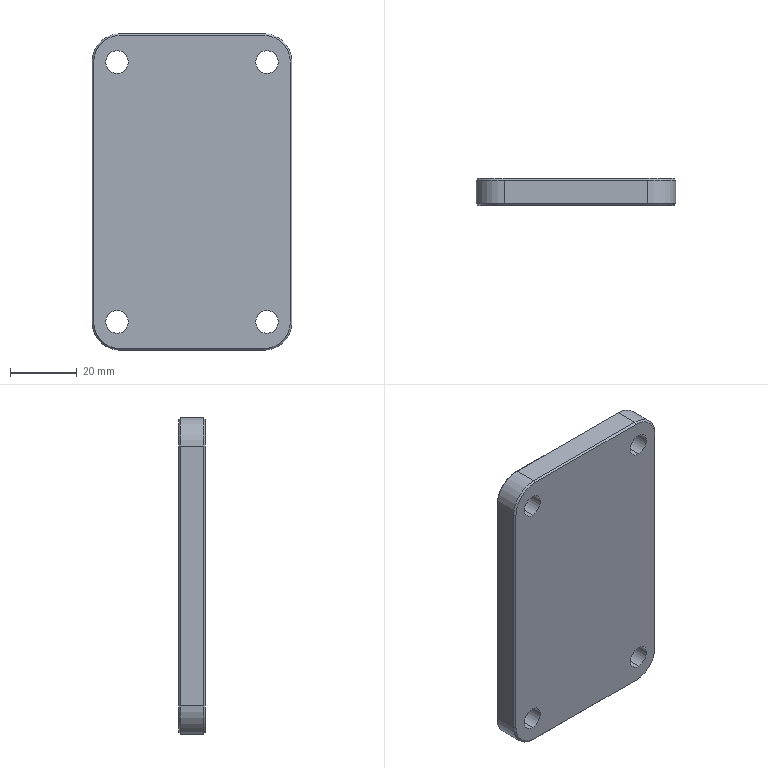Part | SolidWorks | features Chamfer 1, Extrusion 1, Fillet 1, HoleWzd 1 | 1 solid | 34 faces | box 60 x 8 x 95 mm | volume 43868 mm3 | plane 14 | cylinder 12 | cone 8 | commonest cylinder face diameters 6.8 x8 17 x4
STEP:
#1=CARTESIAN_POINT('',(-22.5,0.,-38.1));
#2=VERTEX_POINT('',#1);
#3=CARTESIAN_POINT('',(-22.5,0.,-44.9));
#4=VERTEX_POINT('',#3);
#5=CARTESIAN_POINT('',(-22.5,0.,-41.5));
#6=DIRECTION('',(0.,-1.,0.));
#7=DIRECTION('',(0.,0.,-1.));
#8=AXIS2_PLACEMENT_3D('',#5,#6,#7);
#9=CIRCLE('',#8,3.4);
#10=EDGE_CURVE('',#2,#4,#9,.T.);
#11=ORIENTED_EDGE('',*,*,#10,.F.);
#12=CARTESIAN_POINT('',(-22.5,-8.,-38.1));
#13=VERTEX_POINT('',#12);
#14=CARTESIAN_POINT('',(-22.5,-8.,-38.1));
#15=DIRECTION('',(0.,-1.,0.));
#16=VECTOR('',#15,1000.);
#17=LINE('',#14,#16);
#18=EDGE_CURVE('',#2,#13,#17,.T.);
#19=ORIENTED_EDGE('',*,*,#18,.T.);
#20=CARTESIAN_POINT('',(-22.5,-8.,-44.9));
#21=VERTEX_POINT('',#20);
#22=CARTESIAN_POINT('',(-22.5,-8.,-41.5));
#23=DIRECTION('',(0.,-1.,0.));
#24=DIRECTION('',(0.,0.,-1.));
#25=AXIS2_PLACEMENT_3D('',#22,#23,#24);
#26=CIRCLE('',#25,3.4);
#27=EDGE_CURVE('',#13,#21,#26,.T.);
#28=ORIENTED_EDGE('',*,*,#27,.T.);
#29=CARTESIAN_POINT('',(-22.5,-8.,-44.9));
#30=DIRECTION('',(0.,-1.,0.));
#31=VECTOR('',#30,1000.);
#32=LINE('',#29,#31);
#33=EDGE_CURVE('',#4,#21,#32,.T.);
#34=ORIENTED_EDGE('',*,*,#33,.F.);
#35=EDGE_LOOP('',(#11,#19,#28,#34));
#36=FACE_OUTER_BOUND('',#35,.T.);
#37=CARTESIAN_POINT('',(-22.5,-8.,-41.5));
#38=DIRECTION('',(0.,-1.,0.));
#39=DIRECTION('',(0.,0.,-1.));
#40=AXIS2_PLACEMENT_3D('',#37,#38,#39);
#41=CYLINDRICAL_SURFACE('',#40,3.4);
#42=ADVANCED_FACE('',(#36),#41,.F.);
#43=CARTESIAN_POINT('',(22.5,0.,-38.1));
#44=VERTEX_POINT('',#43);
#45=CARTESIAN_POINT('',(22.5,0.,-44.9));
#46=VERTEX_POINT('',#45);
#47=CARTESIAN_POINT('',(22.5,0.,-41.5));
#48=DIRECTION('',(0.,-1.,0.));
#49=DIRECTION('',(0.,0.,-1.));
#50=AXIS2_PLACEMENT_3D('',#47,#48,#49);
#51=CIRCLE('',#50,3.4);
#52=EDGE_CURVE('',#44,#46,#51,.T.);
#53=ORIENTED_EDGE('',*,*,#52,.F.);
#54=CARTESIAN_POINT('',(22.5,-8.,-38.1));
#55=VERTEX_POINT('',#54);
#56=CARTESIAN_POINT('',(22.5,-8.,-38.1));
#57=DIRECTION('',(0.,-1.,0.));
#58=VECTOR('',#57,1000.);
#59=LINE('',#56,#58);
#60=EDGE_CURVE('',#44,#55,#59,.T.);
#61=ORIENTED_EDGE('',*,*,#60,.T.);
#62=CARTESIAN_POINT('',(22.5,-8.,-44.9));
#63=VERTEX_POINT('',#62);
#64=CARTESIAN_POINT('',(22.5,-8.,-41.5));
#65=DIRECTION('',(0.,-1.,0.));
#66=DIRECTION('',(0.,0.,-1.));
#67=AXIS2_PLACEMENT_3D('',#64,#65,#66);
#68=CIRCLE('',#67,3.4);
#69=EDGE_CURVE('',#55,#63,#68,.T.);
#70=ORIENTED_EDGE('',*,*,#69,.T.);
#71=CARTESIAN_POINT('',(22.5,-8.,-44.9));
#72=DIRECTION('',(0.,-1.,0.));
#73=VECTOR('',#72,1000.);
#74=LINE('',#71,#73);
#75=EDGE_CURVE('',#46,#63,#74,.T.);
#76=ORIENTED_EDGE('',*,*,#75,.F.);
#77=EDGE_LOOP('',(#53,#61,#70,#76));
#78=FACE_OUTER_BOUND('',#77,.T.);
#79=CARTESIAN_POINT('',(22.5,-8.,-41.5));
#80=DIRECTION('',(0.,-1.,0.));
#81=DIRECTION('',(0.,0.,-1.));
#82=AXIS2_PLACEMENT_3D('',#79,#80,#81);
#83=CYLINDRICAL_SURFACE('',#82,3.4);
#84=ADVANCED_FACE('',(#78),#83,.F.);
#85=CARTESIAN_POINT('',(22.5,0.,39.9));
#86=VERTEX_POINT('',#85);
#87=CARTESIAN_POINT('',(22.5,0.,33.1));
#88=VERTEX_POINT('',#87);
#89=CARTESIAN_POINT('',(22.5,0.,36.5));
#90=DIRECTION('',(0.,-1.,0.));
#91=DIRECTION('',(0.,0.,-1.));
#92=AXIS2_PLACEMENT_3D('',#89,#90,#91);
#93=CIRCLE('',#92,3.4);
#94=EDGE_CURVE('',#86,#88,#93,.T.);
#95=ORIENTED_EDGE('',*,*,#94,.F.);
#96=CARTESIAN_POINT('',(22.5,-8.,39.9));
#97=VERTEX_POINT('',#96);
#98=CARTESIAN_POINT('',(22.5,-8.,39.9));
#99=DIRECTION('',(0.,-1.,0.));
#100=VECTOR('',#99,1000.);
#101=LINE('',#98,#100);
#102=EDGE_CURVE('',#86,#97,#101,.T.);
#103=ORIENTED_EDGE('',*,*,#102,.T.);
#104=CARTESIAN_POINT('',(22.5,-8.,33.1));
#105=VERTEX_POINT('',#104);
#106=CARTESIAN_POINT('',(22.5,-8.,36.5));
#107=DIRECTION('',(0.,-1.,0.));
#108=DIRECTION('',(0.,0.,-1.));
#109=AXIS2_PLACEMENT_3D('',#106,#107,#108);
#110=CIRCLE('',#109,3.4);
#111=EDGE_CURVE('',#97,#105,#110,.T.);
#112=ORIENTED_EDGE('',*,*,#111,.T.);
#113=CARTESIAN_POINT('',(22.5,-8.,33.1));
#114=DIRECTION('',(0.,-1.,0.));
#115=VECTOR('',#114,1000.);
#116=LINE('',#113,#115);
#117=EDGE_CURVE('',#88,#105,#116,.T.);
#118=ORIENTED_EDGE('',*,*,#117,.F.);
#119=EDGE_LOOP('',(#95,#103,#112,#118));
#120=FACE_OUTER_BOUND('',#119,.T.);
#121=CARTESIAN_POINT('',(22.5,-8.,36.5));
#122=DIRECTION('',(0.,-1.,0.));
#123=DIRECTION('',(0.,0.,-1.));
#124=AXIS2_PLACEMENT_3D('',#121,#122,#123);
#125=CYLINDRICAL_SURFACE('',#124,3.4);
#126=ADVANCED_FACE('',(#120),#125,.F.);
#127=CARTESIAN_POINT('',(-22.5,0.,39.9));
#128=VERTEX_POINT('',#127);
#129=CARTESIAN_POINT('',(-22.5,0.,33.1));
#130=VERTEX_POINT('',#129);
#131=CARTESIAN_POINT('',(-22.5,0.,36.5));
#132=DIRECTION('',(0.,-1.,0.));
#133=DIRECTION('',(0.,0.,-1.));
#134=AXIS2_PLACEMENT_3D('',#131,#132,#133);
#135=CIRCLE('',#134,3.4);
#136=EDGE_CURVE('',#128,#130,#135,.T.);
#137=ORIENTED_EDGE('',*,*,#136,.F.);
#138=CARTESIAN_POINT('',(-22.5,-8.,39.9));
#139=VERTEX_POINT('',#138);
#140=CARTESIAN_POINT('',(-22.5,-8.,39.9));
#141=DIRECTION('',(0.,-1.,0.));
#142=VECTOR('',#141,1000.);
#143=LINE('',#140,#142);
#144=EDGE_CURVE('',#128,#139,#143,.T.);
#145=ORIENTED_EDGE('',*,*,#144,.T.);
#146=CARTESIAN_POINT('',(-22.5,-8.,33.1));
#147=VERTEX_POINT('',#146);
#148=CARTESIAN_POINT('',(-22.5,-8.,36.5));
#149=DIRECTION('',(0.,-1.,0.));
#150=DIRECTION('',(0.,0.,-1.));
#151=AXIS2_PLACEMENT_3D('',#148,#149,#150);
#152=CIRCLE('',#151,3.4);
#153=EDGE_CURVE('',#139,#147,#152,.T.);
#154=ORIENTED_EDGE('',*,*,#153,.T.);
#155=CARTESIAN_POINT('',(-22.5,-8.,33.1));
#156=DIRECTION('',(0.,-1.,0.));
#157=VECTOR('',#156,1000.);
#158=LINE('',#155,#157);
#159=EDGE_CURVE('',#130,#147,#158,.T.);
#160=ORIENTED_EDGE('',*,*,#159,.F.);
#161=EDGE_LOOP('',(#137,#145,#154,#160));
#162=FACE_OUTER_BOUND('',#161,.T.);
#163=CARTESIAN_POINT('',(-22.5,-8.,36.5));
#164=DIRECTION('',(0.,-1.,0.));
#165=DIRECTION('',(0.,0.,-1.));
#166=AXIS2_PLACEMENT_3D('',#163,#164,#165);
#167=CYLINDRICAL_SURFACE('',#166,3.4);
#168=ADVANCED_FACE('',(#162),#167,.F.);
#169=CARTESIAN_POINT('',(-30.,-7.5,36.5));
#170=VERTEX_POINT('',#169);
#171=CARTESIAN_POINT('',(-30.,-0.5,36.5));
#172=VERTEX_POINT('',#171);
#173=CARTESIAN_POINT('',(-30.,0.,36.5));
#174=DIRECTION('',(0.,1.,0.));
#175=VECTOR('',#174,1000.);
#176=LINE('',#173,#175);
#177=EDGE_CURVE('',#170,#172,#176,.T.);
#178=ORIENTED_EDGE('',*,*,#177,.T.);
#179=CARTESIAN_POINT('',(-30.,-0.5,-41.5));
#180=VERTEX_POINT('',#179);
#181=CARTESIAN_POINT('',(-30.,-0.5,-41.5));
#182=DIRECTION('',(0.,0.,-1.));
#183=VECTOR('',#182,1000.);
#184=LINE('',#181,#183);
#185=EDGE_CURVE('',#172,#180,#184,.T.);
#186=ORIENTED_EDGE('',*,*,#185,.T.);
#187=CARTESIAN_POINT('',(-30.,-7.5,-41.5));
#188=VERTEX_POINT('',#187);
#189=CARTESIAN_POINT('',(-30.,0.,-41.5));
#190=DIRECTION('',(0.,-1.,0.));
#191=VECTOR('',#190,1000.);
#192=LINE('',#189,#191);
#193=EDGE_CURVE('',#180,#188,#192,.T.);
#194=ORIENTED_EDGE('',*,*,#193,.T.);
#195=CARTESIAN_POINT('',(-30.,-7.5,45.));
#196=DIRECTION('',(0.,0.,1.));
#197=VECTOR('',#196,1000.);
#198=LINE('',#195,#197);
#199=EDGE_CURVE('',#188,#170,#198,.T.);
#200=ORIENTED_EDGE('',*,*,#199,.T.);
#201=EDGE_LOOP('',(#178,#186,#194,#200));
#202=FACE_OUTER_BOUND('',#201,.T.);
#203=CARTESIAN_POINT('',(-30.,0.,45.));
#204=DIRECTION('',(-1.,0.,0.));
#205=DIRECTION('',(0.,0.,1.));
#206=AXIS2_PLACEMENT_3D('',#203,#204,#205);
#207=PLANE('',#206);
#208=ADVANCED_FACE('',(#202),#207,.T.);
#209=CARTESIAN_POINT('',(21.5,-7.5,45.));
#210=VERTEX_POINT('',#209);
#211=CARTESIAN_POINT('',(21.5,-0.5,45.));
#212=VERTEX_POINT('',#211);
#213=CARTESIAN_POINT('',(21.5,0.,45.));
#214=DIRECTION('',(0.,1.,0.));
#215=VECTOR('',#214,1000.);
#216=LINE('',#213,#215);
#217=EDGE_CURVE('',#210,#212,#216,.T.);
#218=ORIENTED_EDGE('',*,*,#217,.T.);
#219=CARTESIAN_POINT('',(-21.5,-0.5,45.));
#220=VERTEX_POINT('',#219);
#221=CARTESIAN_POINT('',(-21.5,-0.5,45.));
#222=DIRECTION('',(-1.,0.,0.));
#223=VECTOR('',#222,1000.);
#224=LINE('',#221,#223);
#225=EDGE_CURVE('',#212,#220,#224,.T.);
#226=ORIENTED_EDGE('',*,*,#225,.T.);
#227=CARTESIAN_POINT('',(-21.5,-7.5,45.));
#228=VERTEX_POINT('',#227);
#229=CARTESIAN_POINT('',(-21.5,0.,45.));
#230=DIRECTION('',(0.,-1.,0.));
#231=VECTOR('',#230,1000.);
#232=LINE('',#229,#231);
#233=EDGE_CURVE('',#220,#228,#232,.T.);
#234=ORIENTED_EDGE('',*,*,#233,.T.);
#235=CARTESIAN_POINT('',(30.,-7.5,45.));
#236=DIRECTION('',(1.,0.,0.));
#237=VECTOR('',#236,1000.);
#238=LINE('',#235,#237);
#239=EDGE_CURVE('',#228,#210,#238,.T.);
#240=ORIENTED_EDGE('',*,*,#239,.T.);
#241=EDGE_LOOP('',(#218,#226,#234,#240));
#242=FACE_OUTER_BOUND('',#241,.T.);
#243=CARTESIAN_POINT('',(30.,0.,45.));
#244=DIRECTION('',(0.,0.,1.));
#245=DIRECTION('',(1.,0.,0.));
#246=AXIS2_PLACEMENT_3D('',#243,#244,#245);
#247=PLANE('',#246);
#248=ADVANCED_FACE('',(#242),#247,.T.);
#249=CARTESIAN_POINT('',(30.,-7.5,-41.5));
#250=VERTEX_POINT('',#249);
#251=CARTESIAN_POINT('',(30.,-0.5,-41.5));
#252=VERTEX_POINT('',#251);
#253=CARTESIAN_POINT('',(30.,0.,-41.5));
#254=DIRECTION('',(0.,1.,0.));
#255=VECTOR('',#254,1000.);
#256=LINE('',#253,#255);
#257=EDGE_CURVE('',#250,#252,#256,.T.);
#258=ORIENTED_EDGE('',*,*,#257,.T.);
#259=CARTESIAN_POINT('',(30.,-0.5,36.5));
#260=VERTEX_POINT('',#259);
#261=CARTESIAN_POINT('',(30.,-0.5,36.5));
#262=DIRECTION('',(0.,0.,1.));
#263=VECTOR('',#262,1000.);
#264=LINE('',#261,#263);
#265=EDGE_CURVE('',#252,#260,#264,.T.);
#266=ORIENTED_EDGE('',*,*,#265,.T.);
#267=CARTESIAN_POINT('',(30.,-7.5,36.5));
#268=VERTEX_POINT('',#267);
#269=CARTESIAN_POINT('',(30.,0.,36.5));
#270=DIRECTION('',(0.,-1.,0.));
#271=VECTOR('',#270,1000.);
#272=LINE('',#269,#271);
#273=EDGE_CURVE('',#260,#268,#272,.T.);
#274=ORIENTED_EDGE('',*,*,#273,.T.);
#275=CARTESIAN_POINT('',(30.,-7.5,-50.));
#276=DIRECTION('',(0.,0.,-1.));
#277=VECTOR('',#276,1000.);
#278=LINE('',#275,#277);
#279=EDGE_CURVE('',#268,#250,#278,.T.);
#280=ORIENTED_EDGE('',*,*,#279,.T.);
#281=EDGE_LOOP('',(#258,#266,#274,#280));
#282=FACE_OUTER_BOUND('',#281,.T.);
#283=CARTESIAN_POINT('',(30.,0.,-50.));
#284=DIRECTION('',(1.,0.,0.));
#285=DIRECTION('',(0.,0.,-1.));
#286=AXIS2_PLACEMENT_3D('',#283,#284,#285);
#287=PLANE('',#286);
#288=ADVANCED_FACE('',(#282),#287,.T.);
#289=CARTESIAN_POINT('',(-21.5,-7.5,-50.));
#290=VERTEX_POINT('',#289);
#291=CARTESIAN_POINT('',(-21.5,-0.5,-50.));
#292=VERTEX_POINT('',#291);
#293=CARTESIAN_POINT('',(-21.5,0.,-50.));
#294=DIRECTION('',(0.,1.,0.));
#295=VECTOR('',#294,1000.);
#296=LINE('',#293,#295);
#297=EDGE_CURVE('',#290,#292,#296,.T.);
#298=ORIENTED_EDGE('',*,*,#297,.T.);
#299=CARTESIAN_POINT('',(21.5,-0.5,-50.));
#300=VERTEX_POINT('',#299);
#301=CARTESIAN_POINT('',(21.5,-0.5,-50.));
#302=DIRECTION('',(1.,0.,0.));
#303=VECTOR('',#302,1000.);
#304=LINE('',#301,#303);
#305=EDGE_CURVE('',#292,#300,#304,.T.);
#306=ORIENTED_EDGE('',*,*,#305,.T.);
#307=CARTESIAN_POINT('',(21.5,-7.5,-50.));
#308=VERTEX_POINT('',#307);
#309=CARTESIAN_POINT('',(21.5,0.,-50.));
#310=DIRECTION('',(0.,-1.,0.));
#311=VECTOR('',#310,1000.);
#312=LINE('',#309,#311);
#313=EDGE_CURVE('',#300,#308,#312,.T.);
#314=ORIENTED_EDGE('',*,*,#313,.T.);
#315=CARTESIAN_POINT('',(-30.,-7.5,-50.));
#316=DIRECTION('',(-1.,0.,0.));
#317=VECTOR('',#316,1000.);
#318=LINE('',#315,#317);
#319=EDGE_CURVE('',#308,#290,#318,.T.);
#320=ORIENTED_EDGE('',*,*,#319,.T.);
#321=EDGE_LOOP('',(#298,#306,#314,#320));
#322=FACE_OUTER_BOUND('',#321,.T.);
#323=CARTESIAN_POINT('',(-30.,0.,-50.));
#324=DIRECTION('',(0.,0.,-1.));
#325=DIRECTION('',(-1.,0.,0.));
#326=AXIS2_PLACEMENT_3D('',#323,#324,#325);
#327=PLANE('',#326);
#328=ADVANCED_FACE('',(#322),#327,.T.);
#329=CARTESIAN_POINT('',(21.5,0.,44.5));
#330=VERTEX_POINT('',#329);
#331=CARTESIAN_POINT('',(29.5,0.,36.5));
#332=VERTEX_POINT('',#331);
#333=CARTESIAN_POINT('',(21.5,0.,36.5));
#334=DIRECTION('',(0.,1.,0.));
#335=DIRECTION('',(0.,0.,-1.));
#336=AXIS2_PLACEMENT_3D('',#333,#334,#335);
#337=CIRCLE('',#336,8.);
#338=EDGE_CURVE('',#330,#332,#337,.T.);
#339=ORIENTED_EDGE('',*,*,#338,.T.);
#340=CARTESIAN_POINT('',(29.5,0.,-41.5));
#341=VERTEX_POINT('',#340);
#342=CARTESIAN_POINT('',(29.5,0.,-41.5));
#343=DIRECTION('',(0.,0.,-1.));
#344=VECTOR('',#343,1000.);
#345=LINE('',#342,#344);
#346=EDGE_CURVE('',#332,#341,#345,.T.);
#347=ORIENTED_EDGE('',*,*,#346,.T.);
#348=CARTESIAN_POINT('',(21.5,0.,-49.5));
#349=VERTEX_POINT('',#348);
#350=CARTESIAN_POINT('',(21.5,0.,-41.5));
#351=DIRECTION('',(0.,1.,0.));
#352=DIRECTION('',(0.,0.,-1.));
#353=AXIS2_PLACEMENT_3D('',#350,#351,#352);
#354=CIRCLE('',#353,8.);
#355=EDGE_CURVE('',#341,#349,#354,.T.);
#356=ORIENTED_EDGE('',*,*,#355,.T.);
#357=CARTESIAN_POINT('',(-21.5,0.,-49.5));
#358=VERTEX_POINT('',#357);
#359=CARTESIAN_POINT('',(-21.5,0.,-49.5));
#360=DIRECTION('',(-1.,0.,0.));
#361=VECTOR('',#360,1000.);
#362=LINE('',#359,#361);
#363=EDGE_CURVE('',#349,#358,#362,.T.);
#364=ORIENTED_EDGE('',*,*,#363,.T.);
#365=CARTESIAN_POINT('',(-29.5,0.,-41.5));
#366=VERTEX_POINT('',#365);
#367=CARTESIAN_POINT('',(-21.5,0.,-41.5));
#368=DIRECTION('',(0.,1.,0.));
#369=DIRECTION('',(0.,0.,-1.));
#370=AXIS2_PLACEMENT_3D('',#367,#368,#369);
#371=CIRCLE('',#370,8.);
#372=EDGE_CURVE('',#358,#366,#371,.T.);
#373=ORIENTED_EDGE('',*,*,#372,.T.);
#374=CARTESIAN_POINT('',(-29.5,0.,36.5));
#375=VERTEX_POINT('',#374);
#376=CARTESIAN_POINT('',(-29.5,0.,36.5));
#377=DIRECTION('',(0.,0.,1.));
#378=VECTOR('',#377,1000.);
#379=LINE('',#376,#378);
#380=EDGE_CURVE('',#366,#375,#379,.T.);
#381=ORIENTED_EDGE('',*,*,#380,.T.);
#382=CARTESIAN_POINT('',(-21.5,0.,44.5));
#383=VERTEX_POINT('',#382);
#384=CARTESIAN_POINT('',(-21.5,0.,36.5));
#385=DIRECTION('',(0.,1.,0.));
#386=DIRECTION('',(0.,0.,-1.));
#387=AXIS2_PLACEMENT_3D('',#384,#385,#386);
#388=CIRCLE('',#387,8.);
#389=EDGE_CURVE('',#375,#383,#388,.T.);
#390=ORIENTED_EDGE('',*,*,#389,.T.);
#391=CARTESIAN_POINT('',(21.5,0.,44.5));
#392=DIRECTION('',(1.,0.,0.));
#393=VECTOR('',#392,1000.);
#394=LINE('',#391,#393);
#395=EDGE_CURVE('',#383,#330,#394,.T.);
#396=ORIENTED_EDGE('',*,*,#395,.T.);
#397=EDGE_LOOP('',(#339,#347,#356,#364,#373,#381,#390,#396));
#398=FACE_OUTER_BOUND('',#397,.T.);
#399=CARTESIAN_POINT('',(-22.5,0.,-41.5));
#400=DIRECTION('',(0.,-1.,0.));
#401=DIRECTION('',(0.,0.,-1.));
#402=AXIS2_PLACEMENT_3D('',#399,#400,#401);
#403=CIRCLE('',#402,3.4);
#404=EDGE_CURVE('',#4,#2,#403,.T.);
#405=ORIENTED_EDGE('',*,*,#404,.T.);
#406=ORIENTED_EDGE('',*,*,#10,.T.);
#407=EDGE_LOOP('',(#405,#406));
#408=FACE_BOUND('',#407,.T.);
#409=CARTESIAN_POINT('',(22.5,0.,-41.5));
#410=DIRECTION('',(0.,-1.,0.));
#411=DIRECTION('',(0.,0.,-1.));
#412=AXIS2_PLACEMENT_3D('',#409,#410,#411);
#413=CIRCLE('',#412,3.4);
#414=EDGE_CURVE('',#46,#44,#413,.T.);
#415=ORIENTED_EDGE('',*,*,#414,.T.);
#416=ORIENTED_EDGE('',*,*,#52,.T.);
#417=EDGE_LOOP('',(#415,#416));
#418=FACE_BOUND('',#417,.T.);
#419=CARTESIAN_POINT('',(22.5,0.,36.5));
#420=DIRECTION('',(0.,-1.,0.));
#421=DIRECTION('',(0.,0.,-1.));
#422=AXIS2_PLACEMENT_3D('',#419,#420,#421);
#423=CIRCLE('',#422,3.4);
#424=EDGE_CURVE('',#88,#86,#423,.T.);
#425=ORIENTED_EDGE('',*,*,#424,.T.);
#426=ORIENTED_EDGE('',*,*,#94,.T.);
#427=EDGE_LOOP('',(#425,#426));
#428=FACE_BOUND('',#427,.T.);
#429=CARTESIAN_POINT('',(-22.5,0.,36.5));
#430=DIRECTION('',(0.,-1.,0.));
#431=DIRECTION('',(0.,0.,-1.));
#432=AXIS2_PLACEMENT_3D('',#429,#430,#431);
#433=CIRCLE('',#432,3.4);
#434=EDGE_CURVE('',#130,#128,#433,.T.);
#435=ORIENTED_EDGE('',*,*,#434,.T.);
#436=ORIENTED_EDGE('',*,*,#136,.T.);
#437=EDGE_LOOP('',(#435,#436));
#438=FACE_BOUND('',#437,.T.);
#439=CARTESIAN_POINT('',(0.,0.,0.));
#440=DIRECTION('',(0.,-1.,0.));
#441=DIRECTION('',(0.,0.,-1.));
#442=AXIS2_PLACEMENT_3D('',#439,#440,#441);
#443=PLANE('',#442);
#444=ADVANCED_FACE('',(#398,#408,#418,#428,#438),#443,.F.);
#445=CARTESIAN_POINT('',(21.5,-8.,44.5));
#446=VERTEX_POINT('',#445);
#447=CARTESIAN_POINT('',(-21.5,-8.,44.5));
#448=VERTEX_POINT('',#447);
#449=CARTESIAN_POINT('',(0.,-8.,44.5));
#450=DIRECTION('',(-1.,0.,0.));
#451=VECTOR('',#450,1000.);
#452=LINE('',#449,#451);
#453=EDGE_CURVE('',#446,#448,#452,.T.);
#454=ORIENTED_EDGE('',*,*,#453,.T.);
#455=CARTESIAN_POINT('',(-29.5,-8.,36.5));
#456=VERTEX_POINT('',#455);
#457=CARTESIAN_POINT('',(-21.5,-8.,36.5));
#458=DIRECTION('',(0.,-1.,0.));
#459=DIRECTION('',(0.,0.,-1.));
#460=AXIS2_PLACEMENT_3D('',#457,#458,#459);
#461=CIRCLE('',#460,8.);
#462=EDGE_CURVE('',#448,#456,#461,.T.);
#463=ORIENTED_EDGE('',*,*,#462,.T.);
#464=CARTESIAN_POINT('',(-29.5,-8.,-41.5));
#465=VERTEX_POINT('',#464);
#466=CARTESIAN_POINT('',(-29.5,-8.,0.));
#467=DIRECTION('',(0.,0.,-1.));
#468=VECTOR('',#467,1000.);
#469=LINE('',#466,#468);
#470=EDGE_CURVE('',#456,#465,#469,.T.);
#471=ORIENTED_EDGE('',*,*,#470,.T.);
#472=CARTESIAN_POINT('',(-21.5,-8.,-49.5));
#473=VERTEX_POINT('',#472);
#474=CARTESIAN_POINT('',(-21.5,-8.,-41.5));
#475=DIRECTION('',(0.,-1.,0.));
#476=DIRECTION('',(0.,0.,-1.));
#477=AXIS2_PLACEMENT_3D('',#474,#475,#476);
#478=CIRCLE('',#477,8.);
#479=EDGE_CURVE('',#465,#473,#478,.T.);
#480=ORIENTED_EDGE('',*,*,#479,.T.);
#481=CARTESIAN_POINT('',(21.5,-8.,-49.5));
#482=VERTEX_POINT('',#481);
#483=CARTESIAN_POINT('',(0.,-8.,-49.5));
#484=DIRECTION('',(1.,0.,0.));
#485=VECTOR('',#484,1000.);
#486=LINE('',#483,#485);
#487=EDGE_CURVE('',#473,#482,#486,.T.);
#488=ORIENTED_EDGE('',*,*,#487,.T.);
#489=CARTESIAN_POINT('',(29.5,-8.,-41.5));
#490=VERTEX_POINT('',#489);
#491=CARTESIAN_POINT('',(21.5,-8.,-41.5));
#492=DIRECTION('',(0.,-1.,0.));
#493=DIRECTION('',(0.,0.,-1.));
#494=AXIS2_PLACEMENT_3D('',#491,#492,#493);
#495=CIRCLE('',#494,8.);
#496=EDGE_CURVE('',#482,#490,#495,.T.);
#497=ORIENTED_EDGE('',*,*,#496,.T.);
#498=CARTESIAN_POINT('',(29.5,-8.,36.5));
#499=VERTEX_POINT('',#498);
#500=CARTESIAN_POINT('',(29.5,-8.,0.));
#501=DIRECTION('',(0.,0.,1.));
#502=VECTOR('',#501,1000.);
#503=LINE('',#500,#502);
#504=EDGE_CURVE('',#490,#499,#503,.T.);
#505=ORIENTED_EDGE('',*,*,#504,.T.);
#506=CARTESIAN_POINT('',(21.5,-8.,36.5));
#507=DIRECTION('',(0.,-1.,0.));
#508=DIRECTION('',(0.,0.,-1.));
#509=AXIS2_PLACEMENT_3D('',#506,#507,#508);
#510=CIRCLE('',#509,8.);
#511=EDGE_CURVE('',#499,#446,#510,.T.);
#512=ORIENTED_EDGE('',*,*,#511,.T.);
#513=EDGE_LOOP('',(#454,#463,#471,#480,#488,#497,#505,#512));
#514=FACE_OUTER_BOUND('',#513,.T.);
#515=CARTESIAN_POINT('',(-22.5,-8.,-41.5));
#516=DIRECTION('',(0.,-1.,0.));
#517=DIRECTION('',(0.,0.,-1.));
#518=AXIS2_PLACEMENT_3D('',#515,#516,#517);
#519=CIRCLE('',#518,3.4);
#520=EDGE_CURVE('',#21,#13,#519,.T.);
#521=ORIENTED_EDGE('',*,*,#520,.F.);
#522=ORIENTED_EDGE('',*,*,#27,.F.);
#523=EDGE_LOOP('',(#521,#522));
#524=FACE_BOUND('',#523,.T.);
#525=CARTESIAN_POINT('',(22.5,-8.,-41.5));
#526=DIRECTION('',(0.,-1.,0.));
#527=DIRECTION('',(0.,0.,-1.));
#528=AXIS2_PLACEMENT_3D('',#525,#526,#527);
#529=CIRCLE('',#528,3.4);
#530=EDGE_CURVE('',#63,#55,#529,.T.);
#531=ORIENTED_EDGE('',*,*,#530,.F.);
#532=ORIENTED_EDGE('',*,*,#69,.F.);
#533=EDGE_LOOP('',(#531,#532));
#534=FACE_BOUND('',#533,.T.);
#535=CARTESIAN_POINT('',(22.5,-8.,36.5));
#536=DIRECTION('',(0.,-1.,0.));
#537=DIRECTION('',(0.,0.,-1.));
#538=AXIS2_PLACEMENT_3D('',#535,#536,#537);
#539=CIRCLE('',#538,3.4);
#540=EDGE_CURVE('',#105,#97,#539,.T.);
#541=ORIENTED_EDGE('',*,*,#540,.F.);
#542=ORIENTED_EDGE('',*,*,#111,.F.);
#543=EDGE_LOOP('',(#541,#542));
#544=FACE_BOUND('',#543,.T.);
#545=CARTESIAN_POINT('',(-22.5,-8.,36.5));
#546=DIRECTION('',(0.,-1.,0.));
#547=DIRECTION('',(0.,0.,-1.));
#548=AXIS2_PLACEMENT_3D('',#545,#546,#547);
#549=CIRCLE('',#548,3.4);
#550=EDGE_CURVE('',#147,#139,#549,.T.);
#551=ORIENTED_EDGE('',*,*,#550,.F.);
#552=ORIENTED_EDGE('',*,*,#153,.F.);
#553=EDGE_LOOP('',(#551,#552));
#554=FACE_BOUND('',#553,.T.);
#555=CARTESIAN_POINT('',(0.,-8.,0.));
#556=DIRECTION('',(0.,-1.,0.));
#557=DIRECTION('',(0.,0.,-1.));
#558=AXIS2_PLACEMENT_3D('',#555,#556,#557);
#559=PLANE('',#558);
#560=ADVANCED_FACE('',(#514,#524,#534,#544,#554),#559,.T.);
#561=ORIENTED_EDGE('',*,*,#144,.F.);
#562=ORIENTED_EDGE('',*,*,#434,.F.);
#563=ORIENTED_EDGE('',*,*,#159,.T.);
#564=ORIENTED_EDGE('',*,*,#550,.T.);
#565=EDGE_LOOP('',(#561,#562,#563,#564));
#566=FACE_OUTER_BOUND('',#565,.T.);
#567=CARTESIAN_POINT('',(-22.5,-8.,36.5));
#568=DIRECTION('',(0.,-1.,0.));
#569=DIRECTION('',(0.,0.,-1.));
#570=AXIS2_PLACEMENT_3D('',#567,#568,#569);
#571=CYLINDRICAL_SURFACE('',#570,3.4);
#572=ADVANCED_FACE('',(#566),#571,.F.);
#573=ORIENTED_EDGE('',*,*,#102,.F.);
#574=ORIENTED_EDGE('',*,*,#424,.F.);
#575=ORIENTED_EDGE('',*,*,#117,.T.);
#576=ORIENTED_EDGE('',*,*,#540,.T.);
#577=EDGE_LOOP('',(#573,#574,#575,#576));
#578=FACE_OUTER_BOUND('',#577,.T.);
#579=CARTESIAN_POINT('',(22.5,-8.,36.5));
#580=DIRECTION('',(0.,-1.,0.));
#581=DIRECTION('',(0.,0.,-1.));
#582=AXIS2_PLACEMENT_3D('',#579,#580,#581);
#583=CYLINDRICAL_SURFACE('',#582,3.4);
#584=ADVANCED_FACE('',(#578),#583,.F.);
#585=ORIENTED_EDGE('',*,*,#60,.F.);
#586=ORIENTED_EDGE('',*,*,#414,.F.);
#587=ORIENTED_EDGE('',*,*,#75,.T.);
#588=ORIENTED_EDGE('',*,*,#530,.T.);
#589=EDGE_LOOP('',(#585,#586,#587,#588));
#590=FACE_OUTER_BOUND('',#589,.T.);
#591=CARTESIAN_POINT('',(22.5,-8.,-41.5));
#592=DIRECTION('',(0.,-1.,0.));
#593=DIRECTION('',(0.,0.,-1.));
#594=AXIS2_PLACEMENT_3D('',#591,#592,#593);
#595=CYLINDRICAL_SURFACE('',#594,3.4);
#596=ADVANCED_FACE('',(#590),#595,.F.);
#597=ORIENTED_EDGE('',*,*,#18,.F.);
#598=ORIENTED_EDGE('',*,*,#404,.F.);
#599=ORIENTED_EDGE('',*,*,#33,.T.);
#600=ORIENTED_EDGE('',*,*,#520,.T.);
#601=EDGE_LOOP('',(#597,#598,#599,#600));
#602=FACE_OUTER_BOUND('',#601,.T.);
#603=CARTESIAN_POINT('',(-22.5,-8.,-41.5));
#604=DIRECTION('',(0.,-1.,0.));
#605=DIRECTION('',(0.,0.,-1.));
#606=AXIS2_PLACEMENT_3D('',#603,#604,#605);
#607=CYLINDRICAL_SURFACE('',#606,3.4);
#608=ADVANCED_FACE('',(#602),#607,.F.);
#609=ORIENTED_EDGE('',*,*,#313,.F.);
#610=CARTESIAN_POINT('',(21.5,-0.5,-41.5));
#611=DIRECTION('',(0.,-1.,0.));
#612=DIRECTION('',(0.,0.,-1.));
#613=AXIS2_PLACEMENT_3D('',#610,#611,#612);
#614=CIRCLE('',#613,8.5);
#615=EDGE_CURVE('',#300,#252,#614,.T.);
#616=ORIENTED_EDGE('',*,*,#615,.T.);
#617=ORIENTED_EDGE('',*,*,#257,.F.);
#618=CARTESIAN_POINT('',(21.5,-7.5,-41.5));
#619=DIRECTION('',(0.,1.,0.));
#620=DIRECTION('',(0.,0.,-1.));
#621=AXIS2_PLACEMENT_3D('',#618,#619,#620);
#622=CIRCLE('',#621,8.5);
#623=EDGE_CURVE('',#250,#308,#622,.T.);
#624=ORIENTED_EDGE('',*,*,#623,.T.);
#625=EDGE_LOOP('',(#609,#616,#617,#624));
#626=FACE_OUTER_BOUND('',#625,.T.);
#627=CARTESIAN_POINT('',(21.5,0.,-41.5));
#628=DIRECTION('',(0.,-1.,0.));
#629=DIRECTION('',(0.,0.,-1.));
#630=AXIS2_PLACEMENT_3D('',#627,#628,#629);
#631=CYLINDRICAL_SURFACE('',#630,8.5);
#632=ADVANCED_FACE('',(#626),#631,.T.);
#633=ORIENTED_EDGE('',*,*,#273,.F.);
#634=CARTESIAN_POINT('',(21.5,-0.5,36.5));
#635=DIRECTION('',(0.,-1.,0.));
#636=DIRECTION('',(0.,0.,-1.));
#637=AXIS2_PLACEMENT_3D('',#634,#635,#636);
#638=CIRCLE('',#637,8.5);
#639=EDGE_CURVE('',#260,#212,#638,.T.);
#640=ORIENTED_EDGE('',*,*,#639,.T.);
#641=ORIENTED_EDGE('',*,*,#217,.F.);
#642=CARTESIAN_POINT('',(21.5,-7.5,36.5));
#643=DIRECTION('',(0.,1.,0.));
#644=DIRECTION('',(0.,0.,-1.));
#645=AXIS2_PLACEMENT_3D('',#642,#643,#644);
#646=CIRCLE('',#645,8.5);
#647=EDGE_CURVE('',#210,#268,#646,.T.);
#648=ORIENTED_EDGE('',*,*,#647,.T.);
#649=EDGE_LOOP('',(#633,#640,#641,#648));
#650=FACE_OUTER_BOUND('',#649,.T.);
#651=CARTESIAN_POINT('',(21.5,0.,36.5));
#652=DIRECTION('',(0.,-1.,0.));
#653=DIRECTION('',(0.,0.,-1.));
#654=AXIS2_PLACEMENT_3D('',#651,#652,#653);
#655=CYLINDRICAL_SURFACE('',#654,8.5);
#656=ADVANCED_FACE('',(#650),#655,.T.);
#657=ORIENTED_EDGE('',*,*,#193,.F.);
#658=CARTESIAN_POINT('',(-21.5,-0.5,-41.5));
#659=DIRECTION('',(0.,-1.,0.));
#660=DIRECTION('',(0.,0.,-1.));
#661=AXIS2_PLACEMENT_3D('',#658,#659,#660);
#662=CIRCLE('',#661,8.5);
#663=EDGE_CURVE('',#180,#292,#662,.T.);
#664=ORIENTED_EDGE('',*,*,#663,.T.);
#665=ORIENTED_EDGE('',*,*,#297,.F.);
#666=CARTESIAN_POINT('',(-21.5,-7.5,-41.5));
#667=DIRECTION('',(0.,1.,0.));
#668=DIRECTION('',(0.,0.,-1.));
#669=AXIS2_PLACEMENT_3D('',#666,#667,#668);
#670=CIRCLE('',#669,8.5);
#671=EDGE_CURVE('',#290,#188,#670,.T.);
#672=ORIENTED_EDGE('',*,*,#671,.T.);
#673=EDGE_LOOP('',(#657,#664,#665,#672));
#674=FACE_OUTER_BOUND('',#673,.T.);
#675=CARTESIAN_POINT('',(-21.5,0.,-41.5));
#676=DIRECTION('',(0.,-1.,0.));
#677=DIRECTION('',(0.,0.,-1.));
#678=AXIS2_PLACEMENT_3D('',#675,#676,#677);
#679=CYLINDRICAL_SURFACE('',#678,8.5);
#680=ADVANCED_FACE('',(#674),#679,.T.);
#681=ORIENTED_EDGE('',*,*,#233,.F.);
#682=CARTESIAN_POINT('',(-21.5,-0.5,36.5));
#683=DIRECTION('',(0.,-1.,0.));
#684=DIRECTION('',(0.,0.,-1.));
#685=AXIS2_PLACEMENT_3D('',#682,#683,#684);
#686=CIRCLE('',#685,8.5);
#687=EDGE_CURVE('',#220,#172,#686,.T.);
#688=ORIENTED_EDGE('',*,*,#687,.T.);
#689=ORIENTED_EDGE('',*,*,#177,.F.);
#690=CARTESIAN_POINT('',(-21.5,-7.5,36.5));
#691=DIRECTION('',(0.,1.,0.));
#692=DIRECTION('',(0.,0.,-1.));
#693=AXIS2_PLACEMENT_3D('',#690,#691,#692);
#694=CIRCLE('',#693,8.5);
#695=EDGE_CURVE('',#170,#228,#694,.T.);
#696=ORIENTED_EDGE('',*,*,#695,.T.);
#697=EDGE_LOOP('',(#681,#688,#689,#696));
#698=FACE_OUTER_BOUND('',#697,.T.);
#699=CARTESIAN_POINT('',(-21.5,0.,36.5));
#700=DIRECTION('',(0.,-1.,0.));
#701=DIRECTION('',(0.,0.,-1.));
#702=AXIS2_PLACEMENT_3D('',#699,#700,#701);
#703=CYLINDRICAL_SURFACE('',#702,8.5);
#704=ADVANCED_FACE('',(#698),#703,.T.);
#705=CARTESIAN_POINT('',(-29.5,0.,36.5));
#706=DIRECTION('',(-0.7071,-0.7071,0.));
#707=VECTOR('',#706,1000.);
#708=LINE('',#705,#707);
#709=EDGE_CURVE('',#375,#172,#708,.T.);
#710=ORIENTED_EDGE('',*,*,#709,.F.);
#711=ORIENTED_EDGE('',*,*,#380,.F.);
#712=CARTESIAN_POINT('',(-30.,-0.5,-41.5));
#713=DIRECTION('',(0.7071,0.7071,0.));
#714=VECTOR('',#713,1000.);
#715=LINE('',#712,#714);
#716=EDGE_CURVE('',#180,#366,#715,.T.);
#717=ORIENTED_EDGE('',*,*,#716,.F.);
#718=ORIENTED_EDGE('',*,*,#185,.F.);
#719=EDGE_LOOP('',(#710,#711,#717,#718));
#720=FACE_OUTER_BOUND('',#719,.T.);
#721=CARTESIAN_POINT('',(-30.,-0.5,45.));
#722=DIRECTION('',(-0.7071,0.7071,0.));
#723=DIRECTION('',(0.,0.,1.));
#724=AXIS2_PLACEMENT_3D('',#721,#722,#723);
#725=PLANE('',#724);
#726=ADVANCED_FACE('',(#720),#725,.T.);
#727=ORIENTED_EDGE('',*,*,#716,.T.);
#728=ORIENTED_EDGE('',*,*,#372,.F.);
#729=CARTESIAN_POINT('',(-21.5,-0.5,-50.));
#730=DIRECTION('',(0.,0.7071,0.7071));
#731=VECTOR('',#730,1000.);
#732=LINE('',#729,#731);
#733=EDGE_CURVE('',#292,#358,#732,.T.);
#734=ORIENTED_EDGE('',*,*,#733,.F.);
#735=ORIENTED_EDGE('',*,*,#663,.F.);
#736=EDGE_LOOP('',(#727,#728,#734,#735));
#737=FACE_OUTER_BOUND('',#736,.T.);
#738=CARTESIAN_POINT('',(-21.5,0.,-41.5));
#739=DIRECTION('',(0.,-1.,0.));
#740=DIRECTION('',(0.,0.,-1.));
#741=AXIS2_PLACEMENT_3D('',#738,#739,#740);
#742=CONICAL_SURFACE('',#741,8.,0.7854);
#743=ADVANCED_FACE('',(#737),#742,.T.);
#744=ORIENTED_EDGE('',*,*,#709,.T.);
#745=ORIENTED_EDGE('',*,*,#687,.F.);
#746=CARTESIAN_POINT('',(-21.5,0.,44.5));
#747=DIRECTION('',(0.,-0.7071,0.7071));
#748=VECTOR('',#747,1000.);
#749=LINE('',#746,#748);
#750=EDGE_CURVE('',#383,#220,#749,.T.);
#751=ORIENTED_EDGE('',*,*,#750,.F.);
#752=ORIENTED_EDGE('',*,*,#389,.F.);
#753=EDGE_LOOP('',(#744,#745,#751,#752));
#754=FACE_OUTER_BOUND('',#753,.T.);
#755=CARTESIAN_POINT('',(-21.5,0.,36.5));
#756=DIRECTION('',(0.,-1.,0.));
#757=DIRECTION('',(0.,0.,-1.));
#758=AXIS2_PLACEMENT_3D('',#755,#756,#757);
#759=CONICAL_SURFACE('',#758,8.,0.7854);
#760=ADVANCED_FACE('',(#754),#759,.T.);
#761=ORIENTED_EDGE('',*,*,#733,.T.);
#762=ORIENTED_EDGE('',*,*,#363,.F.);
#763=CARTESIAN_POINT('',(21.5,-0.5,-50.));
#764=DIRECTION('',(0.,0.7071,0.7071));
#765=VECTOR('',#764,1000.);
#766=LINE('',#763,#765);
#767=EDGE_CURVE('',#300,#349,#766,.T.);
#768=ORIENTED_EDGE('',*,*,#767,.F.);
#769=ORIENTED_EDGE('',*,*,#305,.F.);
#770=EDGE_LOOP('',(#761,#762,#768,#769));
#771=FACE_OUTER_BOUND('',#770,.T.);
#772=CARTESIAN_POINT('',(-30.,-0.5,-50.));
#773=DIRECTION('',(0.,0.7071,-0.7071));
#774=DIRECTION('',(-1.,0.,0.));
#775=AXIS2_PLACEMENT_3D('',#772,#773,#774);
#776=PLANE('',#775);
#777=ADVANCED_FACE('',(#771),#776,.T.);
#778=ORIENTED_EDGE('',*,*,#750,.T.);
#779=ORIENTED_EDGE('',*,*,#225,.F.);
#780=CARTESIAN_POINT('',(21.5,0.,44.5));
#781=DIRECTION('',(0.,-0.7071,0.7071));
#782=VECTOR('',#781,1000.);
#783=LINE('',#780,#782);
#784=EDGE_CURVE('',#330,#212,#783,.T.);
#785=ORIENTED_EDGE('',*,*,#784,.F.);
#786=ORIENTED_EDGE('',*,*,#395,.F.);
#787=EDGE_LOOP('',(#778,#779,#785,#786));
#788=FACE_OUTER_BOUND('',#787,.T.);
#789=CARTESIAN_POINT('',(30.,-0.5,45.));
#790=DIRECTION('',(0.,0.7071,0.7071));
#791=DIRECTION('',(1.,0.,0.));
#792=AXIS2_PLACEMENT_3D('',#789,#790,#791);
#793=PLANE('',#792);
#794=ADVANCED_FACE('',(#788),#793,.T.);
#795=ORIENTED_EDGE('',*,*,#767,.T.);
#796=ORIENTED_EDGE('',*,*,#355,.F.);
#797=CARTESIAN_POINT('',(30.,-0.5,-41.5));
#798=DIRECTION('',(-0.7071,0.7071,0.));
#799=VECTOR('',#798,1000.);
#800=LINE('',#797,#799);
#801=EDGE_CURVE('',#252,#341,#800,.T.);
#802=ORIENTED_EDGE('',*,*,#801,.F.);
#803=ORIENTED_EDGE('',*,*,#615,.F.);
#804=EDGE_LOOP('',(#795,#796,#802,#803));
#805=FACE_OUTER_BOUND('',#804,.T.);
#806=CARTESIAN_POINT('',(21.5,0.,-41.5));
#807=DIRECTION('',(0.,-1.,0.));
#808=DIRECTION('',(0.,0.,-1.));
#809=AXIS2_PLACEMENT_3D('',#806,#807,#808);
#810=CONICAL_SURFACE('',#809,8.,0.7854);
#811=ADVANCED_FACE('',(#805),#810,.T.);
#812=ORIENTED_EDGE('',*,*,#784,.T.);
#813=ORIENTED_EDGE('',*,*,#639,.F.);
#814=CARTESIAN_POINT('',(29.5,0.,36.5));
#815=DIRECTION('',(0.7071,-0.7071,0.));
#816=VECTOR('',#815,1000.);
#817=LINE('',#814,#816);
#818=EDGE_CURVE('',#332,#260,#817,.T.);
#819=ORIENTED_EDGE('',*,*,#818,.F.);
#820=ORIENTED_EDGE('',*,*,#338,.F.);
#821=EDGE_LOOP('',(#812,#813,#819,#820));
#822=FACE_OUTER_BOUND('',#821,.T.);
#823=CARTESIAN_POINT('',(21.5,0.,36.5));
#824=DIRECTION('',(0.,-1.,0.));
#825=DIRECTION('',(0.,0.,-1.));
#826=AXIS2_PLACEMENT_3D('',#823,#824,#825);
#827=CONICAL_SURFACE('',#826,8.,0.7854);
#828=ADVANCED_FACE('',(#822),#827,.T.);
#829=ORIENTED_EDGE('',*,*,#801,.T.);
#830=ORIENTED_EDGE('',*,*,#346,.F.);
#831=ORIENTED_EDGE('',*,*,#818,.T.);
#832=ORIENTED_EDGE('',*,*,#265,.F.);
#833=EDGE_LOOP('',(#829,#830,#831,#832));
#834=FACE_OUTER_BOUND('',#833,.T.);
#835=CARTESIAN_POINT('',(30.,-0.5,-50.));
#836=DIRECTION('',(0.7071,0.7071,0.));
#837=DIRECTION('',(0.,0.,-1.));
#838=AXIS2_PLACEMENT_3D('',#835,#836,#837);
#839=PLANE('',#838);
#840=ADVANCED_FACE('',(#834),#839,.T.);
#841=CARTESIAN_POINT('',(21.5,-7.5,-50.));
#842=DIRECTION('',(0.,-0.7071,0.7071));
#843=VECTOR('',#842,1000.);
#844=LINE('',#841,#843);
#845=EDGE_CURVE('',#308,#482,#844,.T.);
#846=ORIENTED_EDGE('',*,*,#845,.F.);
#847=ORIENTED_EDGE('',*,*,#623,.F.);
#848=CARTESIAN_POINT('',(29.5,-8.,-41.5));
#849=DIRECTION('',(0.7071,0.7071,0.));
#850=VECTOR('',#849,1000.);
#851=LINE('',#848,#850);
#852=EDGE_CURVE('',#490,#250,#851,.T.);
#853=ORIENTED_EDGE('',*,*,#852,.F.);
#854=ORIENTED_EDGE('',*,*,#496,.F.);
#855=EDGE_LOOP('',(#846,#847,#853,#854));
#856=FACE_OUTER_BOUND('',#855,.T.);
#857=CARTESIAN_POINT('',(21.5,-8.,-41.5));
#858=DIRECTION('',(0.,1.,0.));
#859=DIRECTION('',(0.,0.,1.));
#860=AXIS2_PLACEMENT_3D('',#857,#858,#859);
#861=CONICAL_SURFACE('',#860,8.,0.7854);
#862=ADVANCED_FACE('',(#856),#861,.T.);
#863=ORIENTED_EDGE('',*,*,#852,.T.);
#864=ORIENTED_EDGE('',*,*,#279,.F.);
#865=CARTESIAN_POINT('',(29.5,-8.,36.5));
#866=DIRECTION('',(0.7071,0.7071,0.));
#867=VECTOR('',#866,1000.);
#868=LINE('',#865,#867);
#869=EDGE_CURVE('',#499,#268,#868,.T.);
#870=ORIENTED_EDGE('',*,*,#869,.F.);
#871=ORIENTED_EDGE('',*,*,#504,.F.);
#872=EDGE_LOOP('',(#863,#864,#870,#871));
#873=FACE_OUTER_BOUND('',#872,.T.);
#874=CARTESIAN_POINT('',(29.5,-8.,0.));
#875=DIRECTION('',(-0.7071,0.7071,0.));
#876=DIRECTION('',(0.,0.,1.));
#877=AXIS2_PLACEMENT_3D('',#874,#875,#876);
#878=PLANE('',#877);
#879=ADVANCED_FACE('',(#873),#878,.F.);
#880=ORIENTED_EDGE('',*,*,#845,.T.);
#881=ORIENTED_EDGE('',*,*,#487,.F.);
#882=CARTESIAN_POINT('',(-21.5,-7.5,-50.));
#883=DIRECTION('',(0.,-0.7071,0.7071));
#884=VECTOR('',#883,1000.);
#885=LINE('',#882,#884);
#886=EDGE_CURVE('',#290,#473,#885,.T.);
#887=ORIENTED_EDGE('',*,*,#886,.F.);
#888=ORIENTED_EDGE('',*,*,#319,.F.);
#889=EDGE_LOOP('',(#880,#881,#887,#888));
#890=FACE_OUTER_BOUND('',#889,.T.);
#891=CARTESIAN_POINT('',(0.,-8.,-49.5));
#892=DIRECTION('',(0.,0.7071,0.7071));
#893=DIRECTION('',(1.,0.,0.));
#894=AXIS2_PLACEMENT_3D('',#891,#892,#893);
#895=PLANE('',#894);
#896=ADVANCED_FACE('',(#890),#895,.F.);
#897=ORIENTED_EDGE('',*,*,#869,.T.);
#898=ORIENTED_EDGE('',*,*,#647,.F.);
#899=CARTESIAN_POINT('',(21.5,-8.,44.5));
#900=DIRECTION('',(0.,0.7071,0.7071));
#901=VECTOR('',#900,1000.);
#902=LINE('',#899,#901);
#903=EDGE_CURVE('',#446,#210,#902,.T.);
#904=ORIENTED_EDGE('',*,*,#903,.F.);
#905=ORIENTED_EDGE('',*,*,#511,.F.);
#906=EDGE_LOOP('',(#897,#898,#904,#905));
#907=FACE_OUTER_BOUND('',#906,.T.);
#908=CARTESIAN_POINT('',(21.5,-8.,36.5));
#909=DIRECTION('',(0.,1.,0.));
#910=DIRECTION('',(0.,0.,1.));
#911=AXIS2_PLACEMENT_3D('',#908,#909,#910);
#912=CONICAL_SURFACE('',#911,8.,0.7854);
#913=ADVANCED_FACE('',(#907),#912,.T.);
#914=ORIENTED_EDGE('',*,*,#886,.T.);
#915=ORIENTED_EDGE('',*,*,#479,.F.);
#916=CARTESIAN_POINT('',(-30.,-7.5,-41.5));
#917=DIRECTION('',(0.7071,-0.7071,0.));
#918=VECTOR('',#917,1000.);
#919=LINE('',#916,#918);
#920=EDGE_CURVE('',#188,#465,#919,.T.);
#921=ORIENTED_EDGE('',*,*,#920,.F.);
#922=ORIENTED_EDGE('',*,*,#671,.F.);
#923=EDGE_LOOP('',(#914,#915,#921,#922));
#924=FACE_OUTER_BOUND('',#923,.T.);
#925=CARTESIAN_POINT('',(-21.5,-8.,-41.5));
#926=DIRECTION('',(0.,1.,0.));
#927=DIRECTION('',(0.,0.,1.));
#928=AXIS2_PLACEMENT_3D('',#925,#926,#927);
#929=CONICAL_SURFACE('',#928,8.,0.7854);
#930=ADVANCED_FACE('',(#924),#929,.T.);
#931=ORIENTED_EDGE('',*,*,#903,.T.);
#932=ORIENTED_EDGE('',*,*,#239,.F.);
#933=CARTESIAN_POINT('',(-21.5,-8.,44.5));
#934=DIRECTION('',(0.,0.7071,0.7071));
#935=VECTOR('',#934,1000.);
#936=LINE('',#933,#935);
#937=EDGE_CURVE('',#448,#228,#936,.T.);
#938=ORIENTED_EDGE('',*,*,#937,.F.);
#939=ORIENTED_EDGE('',*,*,#453,.F.);
#940=EDGE_LOOP('',(#931,#932,#938,#939));
#941=FACE_OUTER_BOUND('',#940,.T.);
#942=CARTESIAN_POINT('',(0.,-8.,44.5));
#943=DIRECTION('',(0.,0.7071,-0.7071));
#944=DIRECTION('',(-1.,0.,0.));
#945=AXIS2_PLACEMENT_3D('',#942,#943,#944);
#946=PLANE('',#945);
#947=ADVANCED_FACE('',(#941),#946,.F.);
#948=ORIENTED_EDGE('',*,*,#920,.T.);
#949=ORIENTED_EDGE('',*,*,#470,.F.);
#950=CARTESIAN_POINT('',(-30.,-7.5,36.5));
#951=DIRECTION('',(0.7071,-0.7071,0.));
#952=VECTOR('',#951,1000.);
#953=LINE('',#950,#952);
#954=EDGE_CURVE('',#170,#456,#953,.T.);
#955=ORIENTED_EDGE('',*,*,#954,.F.);
#956=ORIENTED_EDGE('',*,*,#199,.F.);
#957=EDGE_LOOP('',(#948,#949,#955,#956));
#958=FACE_OUTER_BOUND('',#957,.T.);
#959=CARTESIAN_POINT('',(-29.5,-8.,0.));
#960=DIRECTION('',(0.7071,0.7071,0.));
#961=DIRECTION('',(0.,0.,-1.));
#962=AXIS2_PLACEMENT_3D('',#959,#960,#961);
#963=PLANE('',#962);
#964=ADVANCED_FACE('',(#958),#963,.F.);
#965=ORIENTED_EDGE('',*,*,#937,.T.);
#966=ORIENTED_EDGE('',*,*,#695,.F.);
#967=ORIENTED_EDGE('',*,*,#954,.T.);
#968=ORIENTED_EDGE('',*,*,#462,.F.);
#969=EDGE_LOOP('',(#965,#966,#967,#968));
#970=FACE_OUTER_BOUND('',#969,.T.);
#971=CARTESIAN_POINT('',(-21.5,-8.,36.5));
#972=DIRECTION('',(0.,1.,0.));
#973=DIRECTION('',(0.,0.,1.));
#974=AXIS2_PLACEMENT_3D('',#971,#972,#973);
#975=CONICAL_SURFACE('',#974,8.,0.7854);
#976=ADVANCED_FACE('',(#970),#975,.T.);
#977=CLOSED_SHELL('',(#42,#84,#126,#168,#208,#248,#288,#328,#444,#560,#572,#584,#596,#608,#632,#656,#680,#704,#726,#743,#760,#777,#794,#811,#828,#840,#862,#879,#896,#913,#930,#947,#964,#976));
#978=MANIFOLD_SOLID_BREP('',#977);
#979=CARTESIAN_POINT('',(0.,0.,0.));
#980=DIRECTION('',(0.,0.,1.));
#981=DIRECTION('',(1.,0.,0.));
#982=AXIS2_PLACEMENT_3D('',#979,#980,#981);
#983=(LENGTH_UNIT()NAMED_UNIT(*)SI_UNIT(.MILLI.,.METRE.));
#984=UNCERTAINTY_MEASURE_WITH_UNIT(LENGTH_MEASURE(0.00001),#983,'','');
#985=(NAMED_UNIT(*)PLANE_ANGLE_UNIT()SI_UNIT($,.RADIAN.));
#986=(NAMED_UNIT(*)SI_UNIT($,.STERADIAN.)SOLID_ANGLE_UNIT());
#987=(GEOMETRIC_REPRESENTATION_CONTEXT(3)GLOBAL_UNCERTAINTY_ASSIGNED_CONTEXT((#984))GLOBAL_UNIT_ASSIGNED_CONTEXT((#983,#985,#986))REPRESENTATION_CONTEXT('',''));
#988=ADVANCED_BREP_SHAPE_REPRESENTATION('',(#978,#982),#987);